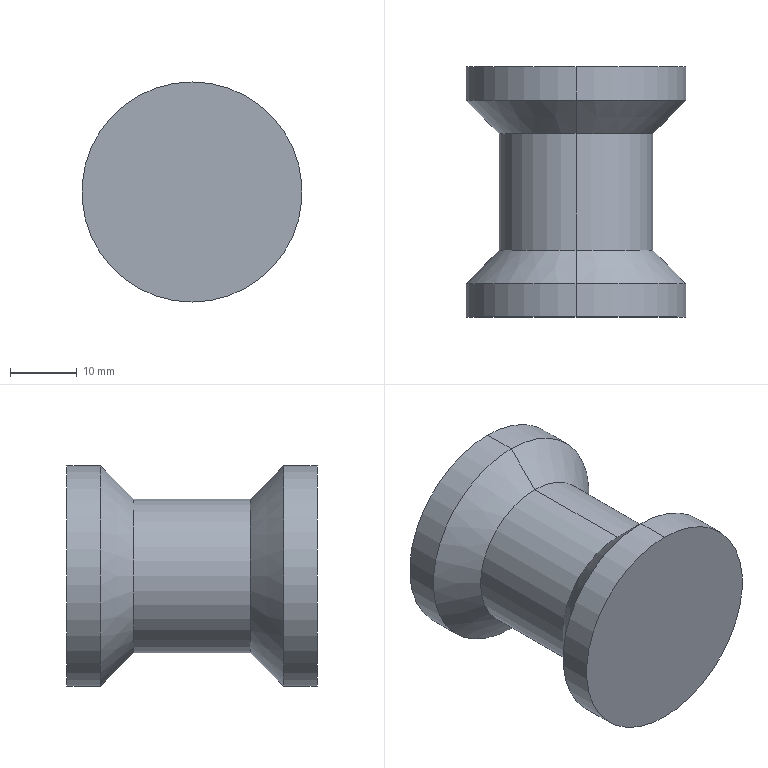Part | SolidWorks | features Chamfer 1, Extrusion 1, RevCut 1 | 1 solid | 12 faces | box 33 x 37.5 x 33 mm | volume 22047 mm3 | cylinder 6 | cone 4 | plane 2 | commonest cylinder face diameters 33 x4 23 x2
STEP:
#1=CARTESIAN_POINT('',(0.,27.5,-11.5));
#2=VERTEX_POINT('',#1);
#3=CARTESIAN_POINT('',(0.,27.5,11.5));
#4=VERTEX_POINT('',#3);
#5=CARTESIAN_POINT('',(0.,27.5,0.));
#6=DIRECTION('',(0.,-1.,0.));
#7=DIRECTION('',(0.,0.,-1.));
#8=AXIS2_PLACEMENT_3D('',#5,#6,#7);
#9=CIRCLE('',#8,11.5);
#10=EDGE_CURVE('',#2,#4,#9,.T.);
#11=ORIENTED_EDGE('',*,*,#10,.F.);
#12=CARTESIAN_POINT('',(0.,32.5,-16.5));
#13=VERTEX_POINT('',#12);
#14=CARTESIAN_POINT('',(0.,32.5,-16.5));
#15=DIRECTION('',(0.,0.7071,-0.7071));
#16=VECTOR('',#15,1000.);
#17=LINE('',#14,#16);
#18=EDGE_CURVE('',#2,#13,#17,.T.);
#19=ORIENTED_EDGE('',*,*,#18,.T.);
#20=CARTESIAN_POINT('',(0.,32.5,16.5));
#21=VERTEX_POINT('',#20);
#22=CARTESIAN_POINT('',(0.,32.5,0.));
#23=DIRECTION('',(0.,1.,0.));
#24=DIRECTION('',(0.,0.,1.));
#25=AXIS2_PLACEMENT_3D('',#22,#23,#24);
#26=CIRCLE('',#25,16.5);
#27=EDGE_CURVE('',#21,#13,#26,.T.);
#28=ORIENTED_EDGE('',*,*,#27,.F.);
#29=CARTESIAN_POINT('',(0.,32.5,16.5));
#30=DIRECTION('',(0.,0.7071,0.7071));
#31=VECTOR('',#30,1000.);
#32=LINE('',#29,#31);
#33=EDGE_CURVE('',#4,#21,#32,.T.);
#34=ORIENTED_EDGE('',*,*,#33,.F.);
#35=EDGE_LOOP('',(#11,#19,#28,#34));
#36=FACE_OUTER_BOUND('',#35,.T.);
#37=CARTESIAN_POINT('',(0.,32.5,0.));
#38=DIRECTION('',(0.,1.,0.));
#39=DIRECTION('',(0.,0.,1.));
#40=AXIS2_PLACEMENT_3D('',#37,#38,#39);
#41=CONICAL_SURFACE('',#40,16.5,0.7854);
#42=ADVANCED_FACE('',(#36),#41,.T.);
#43=CARTESIAN_POINT('',(0.,10.,11.5));
#44=VERTEX_POINT('',#43);
#45=CARTESIAN_POINT('',(0.,10.,-11.5));
#46=VERTEX_POINT('',#45);
#47=CARTESIAN_POINT('',(0.,10.,0.));
#48=DIRECTION('',(0.,1.,0.));
#49=DIRECTION('',(0.,0.,1.));
#50=AXIS2_PLACEMENT_3D('',#47,#48,#49);
#51=CIRCLE('',#50,11.5);
#52=EDGE_CURVE('',#44,#46,#51,.T.);
#53=ORIENTED_EDGE('',*,*,#52,.F.);
#54=CARTESIAN_POINT('',(0.,5.,16.5));
#55=VERTEX_POINT('',#54);
#56=CARTESIAN_POINT('',(0.,10.,11.5));
#57=DIRECTION('',(0.,-0.7071,0.7071));
#58=VECTOR('',#57,1000.);
#59=LINE('',#56,#58);
#60=EDGE_CURVE('',#44,#55,#59,.T.);
#61=ORIENTED_EDGE('',*,*,#60,.T.);
#62=CARTESIAN_POINT('',(0.,5.,-16.5));
#63=VERTEX_POINT('',#62);
#64=CARTESIAN_POINT('',(0.,5.,0.));
#65=DIRECTION('',(0.,1.,0.));
#66=DIRECTION('',(0.,0.,1.));
#67=AXIS2_PLACEMENT_3D('',#64,#65,#66);
#68=CIRCLE('',#67,16.5);
#69=EDGE_CURVE('',#55,#63,#68,.T.);
#70=ORIENTED_EDGE('',*,*,#69,.T.);
#71=CARTESIAN_POINT('',(0.,10.,-11.5));
#72=DIRECTION('',(0.,-0.7071,-0.7071));
#73=VECTOR('',#72,1000.);
#74=LINE('',#71,#73);
#75=EDGE_CURVE('',#46,#63,#74,.T.);
#76=ORIENTED_EDGE('',*,*,#75,.F.);
#77=EDGE_LOOP('',(#53,#61,#70,#76));
#78=FACE_OUTER_BOUND('',#77,.T.);
#79=CARTESIAN_POINT('',(0.,10.,0.));
#80=DIRECTION('',(0.,-1.,0.));
#81=DIRECTION('',(0.,0.,-1.));
#82=AXIS2_PLACEMENT_3D('',#79,#80,#81);
#83=CONICAL_SURFACE('',#82,11.5,0.7854);
#84=ADVANCED_FACE('',(#78),#83,.T.);
#85=CARTESIAN_POINT('',(0.,37.5,16.5));
#86=VERTEX_POINT('',#85);
#87=CARTESIAN_POINT('',(0.,37.5,-16.5));
#88=VERTEX_POINT('',#87);
#89=CARTESIAN_POINT('',(0.,37.5,0.));
#90=DIRECTION('',(0.,1.,0.));
#91=DIRECTION('',(0.,0.,1.));
#92=AXIS2_PLACEMENT_3D('',#89,#90,#91);
#93=CIRCLE('',#92,16.5);
#94=EDGE_CURVE('',#86,#88,#93,.T.);
#95=ORIENTED_EDGE('',*,*,#94,.F.);
#96=CARTESIAN_POINT('',(0.,37.5,16.5));
#97=DIRECTION('',(0.,-1.,0.));
#98=VECTOR('',#97,1000.);
#99=LINE('',#96,#98);
#100=EDGE_CURVE('',#86,#21,#99,.T.);
#101=ORIENTED_EDGE('',*,*,#100,.T.);
#102=ORIENTED_EDGE('',*,*,#27,.T.);
#103=CARTESIAN_POINT('',(0.,37.5,-16.5));
#104=DIRECTION('',(0.,-1.,0.));
#105=VECTOR('',#104,1000.);
#106=LINE('',#103,#105);
#107=EDGE_CURVE('',#88,#13,#106,.T.);
#108=ORIENTED_EDGE('',*,*,#107,.F.);
#109=EDGE_LOOP('',(#95,#101,#102,#108));
#110=FACE_OUTER_BOUND('',#109,.T.);
#111=CARTESIAN_POINT('',(0.,37.5,0.));
#112=DIRECTION('',(0.,-1.,0.));
#113=DIRECTION('',(0.,0.,-1.));
#114=AXIS2_PLACEMENT_3D('',#111,#112,#113);
#115=CYLINDRICAL_SURFACE('',#114,16.5);
#116=ADVANCED_FACE('',(#110),#115,.T.);
#117=ORIENTED_EDGE('',*,*,#52,.T.);
#118=CARTESIAN_POINT('',(0.,35.015,-11.5));
#119=DIRECTION('',(0.,1.,0.));
#120=VECTOR('',#119,1000.);
#121=LINE('',#118,#120);
#122=EDGE_CURVE('',#46,#2,#121,.T.);
#123=ORIENTED_EDGE('',*,*,#122,.T.);
#124=ORIENTED_EDGE('',*,*,#10,.T.);
#125=CARTESIAN_POINT('',(0.,35.015,11.5));
#126=DIRECTION('',(0.,1.,0.));
#127=VECTOR('',#126,1000.);
#128=LINE('',#125,#127);
#129=EDGE_CURVE('',#44,#4,#128,.T.);
#130=ORIENTED_EDGE('',*,*,#129,.F.);
#131=EDGE_LOOP('',(#117,#123,#124,#130));
#132=FACE_OUTER_BOUND('',#131,.T.);
#133=CARTESIAN_POINT('',(0.,35.015,0.));
#134=DIRECTION('',(0.,1.,0.));
#135=DIRECTION('',(0.,0.,1.));
#136=AXIS2_PLACEMENT_3D('',#133,#134,#135);
#137=CYLINDRICAL_SURFACE('',#136,11.5);
#138=ADVANCED_FACE('',(#132),#137,.T.);
#139=ORIENTED_EDGE('',*,*,#69,.F.);
#140=CARTESIAN_POINT('',(0.,0.,16.5));
#141=VERTEX_POINT('',#140);
#142=CARTESIAN_POINT('',(0.,37.5,16.5));
#143=DIRECTION('',(0.,-1.,0.));
#144=VECTOR('',#143,1000.);
#145=LINE('',#142,#144);
#146=EDGE_CURVE('',#55,#141,#145,.T.);
#147=ORIENTED_EDGE('',*,*,#146,.T.);
#148=CARTESIAN_POINT('',(0.,0.,-16.5));
#149=VERTEX_POINT('',#148);
#150=CARTESIAN_POINT('',(0.,0.,0.));
#151=DIRECTION('',(0.,1.,0.));
#152=DIRECTION('',(0.,0.,1.));
#153=AXIS2_PLACEMENT_3D('',#150,#151,#152);
#154=CIRCLE('',#153,16.5);
#155=EDGE_CURVE('',#141,#149,#154,.T.);
#156=ORIENTED_EDGE('',*,*,#155,.T.);
#157=CARTESIAN_POINT('',(0.,37.5,-16.5));
#158=DIRECTION('',(0.,-1.,0.));
#159=VECTOR('',#158,1000.);
#160=LINE('',#157,#159);
#161=EDGE_CURVE('',#63,#149,#160,.T.);
#162=ORIENTED_EDGE('',*,*,#161,.F.);
#163=EDGE_LOOP('',(#139,#147,#156,#162));
#164=FACE_OUTER_BOUND('',#163,.T.);
#165=CARTESIAN_POINT('',(0.,37.5,0.));
#166=DIRECTION('',(0.,-1.,0.));
#167=DIRECTION('',(0.,0.,-1.));
#168=AXIS2_PLACEMENT_3D('',#165,#166,#167);
#169=CYLINDRICAL_SURFACE('',#168,16.5);
#170=ADVANCED_FACE('',(#164),#169,.T.);
#171=ORIENTED_EDGE('',*,*,#146,.F.);
#172=CARTESIAN_POINT('',(0.,5.,0.));
#173=DIRECTION('',(0.,1.,0.));
#174=DIRECTION('',(0.,0.,1.));
#175=AXIS2_PLACEMENT_3D('',#172,#173,#174);
#176=CIRCLE('',#175,16.5);
#177=EDGE_CURVE('',#63,#55,#176,.T.);
#178=ORIENTED_EDGE('',*,*,#177,.F.);
#179=ORIENTED_EDGE('',*,*,#161,.T.);
#180=CARTESIAN_POINT('',(0.,0.,0.));
#181=DIRECTION('',(0.,1.,0.));
#182=DIRECTION('',(0.,0.,1.));
#183=AXIS2_PLACEMENT_3D('',#180,#181,#182);
#184=CIRCLE('',#183,16.5);
#185=EDGE_CURVE('',#149,#141,#184,.T.);
#186=ORIENTED_EDGE('',*,*,#185,.T.);
#187=EDGE_LOOP('',(#171,#178,#179,#186));
#188=FACE_OUTER_BOUND('',#187,.T.);
#189=CARTESIAN_POINT('',(0.,37.5,0.));
#190=DIRECTION('',(0.,-1.,0.));
#191=DIRECTION('',(0.,0.,-1.));
#192=AXIS2_PLACEMENT_3D('',#189,#190,#191);
#193=CYLINDRICAL_SURFACE('',#192,16.5);
#194=ADVANCED_FACE('',(#188),#193,.T.);
#195=ORIENTED_EDGE('',*,*,#185,.F.);
#196=ORIENTED_EDGE('',*,*,#155,.F.);
#197=EDGE_LOOP('',(#195,#196));
#198=FACE_OUTER_BOUND('',#197,.T.);
#199=CARTESIAN_POINT('',(0.,0.,0.));
#200=DIRECTION('',(0.,1.,0.));
#201=DIRECTION('',(0.,0.,1.));
#202=AXIS2_PLACEMENT_3D('',#199,#200,#201);
#203=PLANE('',#202);
#204=ADVANCED_FACE('',(#198),#203,.F.);
#205=ORIENTED_EDGE('',*,*,#122,.F.);
#206=CARTESIAN_POINT('',(0.,10.,0.));
#207=DIRECTION('',(0.,1.,0.));
#208=DIRECTION('',(0.,0.,1.));
#209=AXIS2_PLACEMENT_3D('',#206,#207,#208);
#210=CIRCLE('',#209,11.5);
#211=EDGE_CURVE('',#46,#44,#210,.T.);
#212=ORIENTED_EDGE('',*,*,#211,.T.);
#213=ORIENTED_EDGE('',*,*,#129,.T.);
#214=CARTESIAN_POINT('',(0.,27.5,0.));
#215=DIRECTION('',(0.,-1.,0.));
#216=DIRECTION('',(0.,0.,-1.));
#217=AXIS2_PLACEMENT_3D('',#214,#215,#216);
#218=CIRCLE('',#217,11.5);
#219=EDGE_CURVE('',#4,#2,#218,.T.);
#220=ORIENTED_EDGE('',*,*,#219,.T.);
#221=EDGE_LOOP('',(#205,#212,#213,#220));
#222=FACE_OUTER_BOUND('',#221,.T.);
#223=CARTESIAN_POINT('',(0.,35.015,0.));
#224=DIRECTION('',(0.,1.,0.));
#225=DIRECTION('',(0.,0.,1.));
#226=AXIS2_PLACEMENT_3D('',#223,#224,#225);
#227=CYLINDRICAL_SURFACE('',#226,11.5);
#228=ADVANCED_FACE('',(#222),#227,.T.);
#229=CARTESIAN_POINT('',(0.,37.5,0.));
#230=DIRECTION('',(0.,1.,0.));
#231=DIRECTION('',(0.,0.,1.));
#232=AXIS2_PLACEMENT_3D('',#229,#230,#231);
#233=CIRCLE('',#232,16.5);
#234=EDGE_CURVE('',#88,#86,#233,.T.);
#235=ORIENTED_EDGE('',*,*,#234,.T.);
#236=ORIENTED_EDGE('',*,*,#94,.T.);
#237=EDGE_LOOP('',(#235,#236));
#238=FACE_OUTER_BOUND('',#237,.T.);
#239=CARTESIAN_POINT('',(0.,37.5,0.));
#240=DIRECTION('',(0.,1.,0.));
#241=DIRECTION('',(0.,0.,1.));
#242=AXIS2_PLACEMENT_3D('',#239,#240,#241);
#243=PLANE('',#242);
#244=ADVANCED_FACE('',(#238),#243,.T.);
#245=ORIENTED_EDGE('',*,*,#100,.F.);
#246=ORIENTED_EDGE('',*,*,#234,.F.);
#247=ORIENTED_EDGE('',*,*,#107,.T.);
#248=CARTESIAN_POINT('',(0.,32.5,0.));
#249=DIRECTION('',(0.,1.,0.));
#250=DIRECTION('',(0.,0.,1.));
#251=AXIS2_PLACEMENT_3D('',#248,#249,#250);
#252=CIRCLE('',#251,16.5);
#253=EDGE_CURVE('',#13,#21,#252,.T.);
#254=ORIENTED_EDGE('',*,*,#253,.T.);
#255=EDGE_LOOP('',(#245,#246,#247,#254));
#256=FACE_OUTER_BOUND('',#255,.T.);
#257=CARTESIAN_POINT('',(0.,37.5,0.));
#258=DIRECTION('',(0.,-1.,0.));
#259=DIRECTION('',(0.,0.,-1.));
#260=AXIS2_PLACEMENT_3D('',#257,#258,#259);
#261=CYLINDRICAL_SURFACE('',#260,16.5);
#262=ADVANCED_FACE('',(#256),#261,.T.);
#263=ORIENTED_EDGE('',*,*,#60,.F.);
#264=ORIENTED_EDGE('',*,*,#211,.F.);
#265=ORIENTED_EDGE('',*,*,#75,.T.);
#266=ORIENTED_EDGE('',*,*,#177,.T.);
#267=EDGE_LOOP('',(#263,#264,#265,#266));
#268=FACE_OUTER_BOUND('',#267,.T.);
#269=CARTESIAN_POINT('',(0.,10.,0.));
#270=DIRECTION('',(0.,-1.,0.));
#271=DIRECTION('',(0.,0.,-1.));
#272=AXIS2_PLACEMENT_3D('',#269,#270,#271);
#273=CONICAL_SURFACE('',#272,11.5,0.7854);
#274=ADVANCED_FACE('',(#268),#273,.T.);
#275=ORIENTED_EDGE('',*,*,#18,.F.);
#276=ORIENTED_EDGE('',*,*,#219,.F.);
#277=ORIENTED_EDGE('',*,*,#33,.T.);
#278=ORIENTED_EDGE('',*,*,#253,.F.);
#279=EDGE_LOOP('',(#275,#276,#277,#278));
#280=FACE_OUTER_BOUND('',#279,.T.);
#281=CARTESIAN_POINT('',(0.,32.5,0.));
#282=DIRECTION('',(0.,1.,0.));
#283=DIRECTION('',(0.,0.,1.));
#284=AXIS2_PLACEMENT_3D('',#281,#282,#283);
#285=CONICAL_SURFACE('',#284,16.5,0.7854);
#286=ADVANCED_FACE('',(#280),#285,.T.);
#287=CLOSED_SHELL('',(#42,#84,#116,#138,#170,#194,#204,#228,#244,#262,#274,#286));
#288=MANIFOLD_SOLID_BREP('',#287);
#289=CARTESIAN_POINT('',(0.,0.,0.));
#290=DIRECTION('',(0.,0.,1.));
#291=DIRECTION('',(1.,0.,0.));
#292=AXIS2_PLACEMENT_3D('',#289,#290,#291);
#293=(LENGTH_UNIT()NAMED_UNIT(*)SI_UNIT(.MILLI.,.METRE.));
#294=UNCERTAINTY_MEASURE_WITH_UNIT(LENGTH_MEASURE(0.00001),#293,'','');
#295=(NAMED_UNIT(*)PLANE_ANGLE_UNIT()SI_UNIT($,.RADIAN.));
#296=(NAMED_UNIT(*)SI_UNIT($,.STERADIAN.)SOLID_ANGLE_UNIT());
#297=(GEOMETRIC_REPRESENTATION_CONTEXT(3)GLOBAL_UNCERTAINTY_ASSIGNED_CONTEXT((#294))GLOBAL_UNIT_ASSIGNED_CONTEXT((#293,#295,#296))REPRESENTATION_CONTEXT('',''));
#298=ADVANCED_BREP_SHAPE_REPRESENTATION('',(#288,#292),#297);